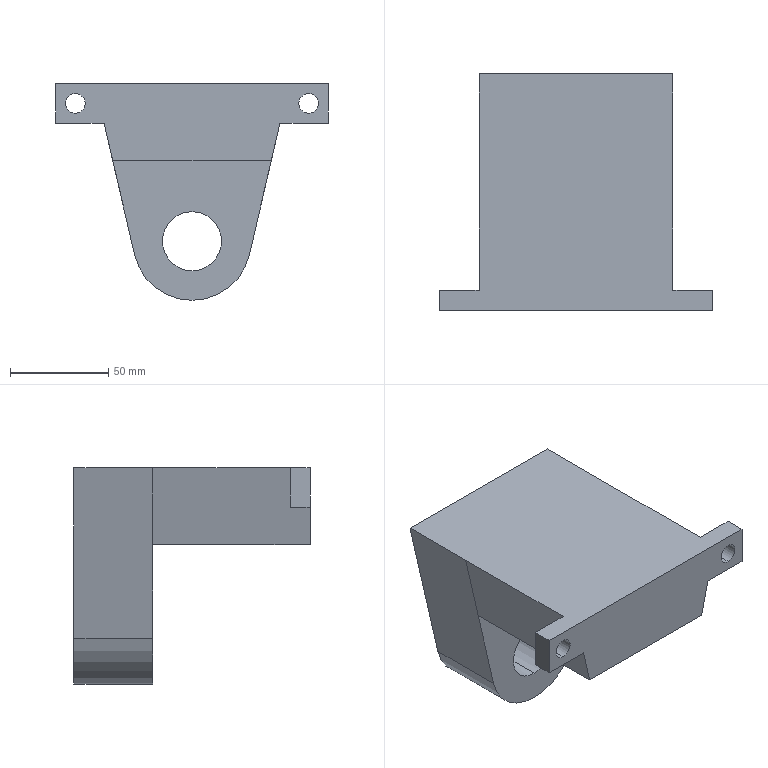Part | SolidWorks | features BaseBody 1 | 1 solid | 25 faces | box 138.517 x 120 x 109.993 mm | volume 571156 mm3 | plane 17 | cylinder 8 | commonest cylinder face diameters 10 x4 30 x2 59.986 x2
STEP:
#1=CARTESIAN_POINT('',(418.218,7.138,-275.));
#2=VERTEX_POINT('',#1);
#3=CARTESIAN_POINT('',(418.218,7.138,-285.));
#4=VERTEX_POINT('',#3);
#5=CARTESIAN_POINT('',(418.218,7.138,-280.));
#6=DIRECTION('',(0.,-1.,0.));
#7=DIRECTION('',(0.,0.,1.));
#8=AXIS2_PLACEMENT_3D('',#5,#6,#7);
#9=CIRCLE('',#8,5.);
#10=EDGE_CURVE('',#2,#4,#9,.T.);
#11=ORIENTED_EDGE('',*,*,#10,.T.);
#12=CARTESIAN_POINT('',(418.218,17.138,-285.));
#13=VERTEX_POINT('',#12);
#14=CARTESIAN_POINT('',(418.218,-2.862,-285.));
#15=DIRECTION('',(0.,1.,0.));
#16=VECTOR('',#15,1000.);
#17=LINE('',#14,#16);
#18=EDGE_CURVE('',#4,#13,#17,.T.);
#19=ORIENTED_EDGE('',*,*,#18,.T.);
#20=CARTESIAN_POINT('',(418.218,17.138,-275.));
#21=VERTEX_POINT('',#20);
#22=CARTESIAN_POINT('',(418.218,17.138,-280.));
#23=DIRECTION('',(0.,1.,0.));
#24=DIRECTION('',(0.,0.,1.));
#25=AXIS2_PLACEMENT_3D('',#22,#23,#24);
#26=CIRCLE('',#25,5.);
#27=EDGE_CURVE('',#13,#21,#26,.T.);
#28=ORIENTED_EDGE('',*,*,#27,.T.);
#29=CARTESIAN_POINT('',(418.218,-2.862,-275.));
#30=DIRECTION('',(0.,1.,0.));
#31=VECTOR('',#30,1000.);
#32=LINE('',#29,#31);
#33=EDGE_CURVE('',#2,#21,#32,.T.);
#34=ORIENTED_EDGE('',*,*,#33,.F.);
#35=EDGE_LOOP('',(#11,#19,#28,#34));
#36=FACE_OUTER_BOUND('',#35,.T.);
#37=CARTESIAN_POINT('',(418.218,-2.862,-280.));
#38=DIRECTION('',(0.,1.,0.));
#39=DIRECTION('',(0.,0.,1.));
#40=AXIS2_PLACEMENT_3D('',#37,#38,#39);
#41=CYLINDRICAL_SURFACE('',#40,5.);
#42=ADVANCED_FACE('',(#36),#41,.F.);
#43=CARTESIAN_POINT('',(299.701,7.138,-275.));
#44=VERTEX_POINT('',#43);
#45=CARTESIAN_POINT('',(299.701,7.138,-285.));
#46=VERTEX_POINT('',#45);
#47=CARTESIAN_POINT('',(299.701,7.138,-280.));
#48=DIRECTION('',(0.,-1.,0.));
#49=DIRECTION('',(0.,0.,1.));
#50=AXIS2_PLACEMENT_3D('',#47,#48,#49);
#51=CIRCLE('',#50,5.);
#52=EDGE_CURVE('',#44,#46,#51,.T.);
#53=ORIENTED_EDGE('',*,*,#52,.T.);
#54=CARTESIAN_POINT('',(299.701,17.138,-285.));
#55=VERTEX_POINT('',#54);
#56=CARTESIAN_POINT('',(299.701,-2.862,-285.));
#57=DIRECTION('',(0.,1.,0.));
#58=VECTOR('',#57,1000.);
#59=LINE('',#56,#58);
#60=EDGE_CURVE('',#46,#55,#59,.T.);
#61=ORIENTED_EDGE('',*,*,#60,.T.);
#62=CARTESIAN_POINT('',(299.701,17.138,-275.));
#63=VERTEX_POINT('',#62);
#64=CARTESIAN_POINT('',(299.701,17.138,-280.));
#65=DIRECTION('',(0.,1.,0.));
#66=DIRECTION('',(0.,0.,1.));
#67=AXIS2_PLACEMENT_3D('',#64,#65,#66);
#68=CIRCLE('',#67,5.);
#69=EDGE_CURVE('',#55,#63,#68,.T.);
#70=ORIENTED_EDGE('',*,*,#69,.T.);
#71=CARTESIAN_POINT('',(299.701,-2.862,-275.));
#72=DIRECTION('',(0.,1.,0.));
#73=VECTOR('',#72,1000.);
#74=LINE('',#71,#73);
#75=EDGE_CURVE('',#44,#63,#74,.T.);
#76=ORIENTED_EDGE('',*,*,#75,.F.);
#77=EDGE_LOOP('',(#53,#61,#70,#76));
#78=FACE_OUTER_BOUND('',#77,.T.);
#79=CARTESIAN_POINT('',(299.701,-2.862,-280.));
#80=DIRECTION('',(0.,1.,0.));
#81=DIRECTION('',(0.,0.,1.));
#82=AXIS2_PLACEMENT_3D('',#79,#80,#81);
#83=CYLINDRICAL_SURFACE('',#82,5.);
#84=ADVANCED_FACE('',(#78),#83,.F.);
#85=CARTESIAN_POINT('',(358.959,127.138,-379.993));
#86=VERTEX_POINT('',#85);
#87=CARTESIAN_POINT('',(329.736,127.138,-356.749));
#88=VERTEX_POINT('',#87);
#89=CARTESIAN_POINT('',(358.959,127.138,-350.));
#90=DIRECTION('',(0.,1.,0.));
#91=DIRECTION('',(0.,0.,1.));
#92=AXIS2_PLACEMENT_3D('',#89,#90,#91);
#93=CIRCLE('',#92,29.993);
#94=EDGE_CURVE('',#86,#88,#93,.T.);
#95=ORIENTED_EDGE('',*,*,#94,.F.);
#96=CARTESIAN_POINT('',(358.959,87.138,-379.993));
#97=VERTEX_POINT('',#96);
#98=CARTESIAN_POINT('',(358.959,127.138,-379.993));
#99=DIRECTION('',(0.,-1.,0.));
#100=VECTOR('',#99,1000.);
#101=LINE('',#98,#100);
#102=EDGE_CURVE('',#86,#97,#101,.T.);
#103=ORIENTED_EDGE('',*,*,#102,.T.);
#104=CARTESIAN_POINT('',(329.736,87.138,-356.749));
#105=VERTEX_POINT('',#104);
#106=CARTESIAN_POINT('',(358.959,87.138,-350.));
#107=DIRECTION('',(0.,1.,0.));
#108=DIRECTION('',(0.,0.,1.));
#109=AXIS2_PLACEMENT_3D('',#106,#107,#108);
#110=CIRCLE('',#109,29.993);
#111=EDGE_CURVE('',#97,#105,#110,.T.);
#112=ORIENTED_EDGE('',*,*,#111,.T.);
#113=CARTESIAN_POINT('',(329.736,127.138,-356.749));
#114=DIRECTION('',(0.,-1.,0.));
#115=VECTOR('',#114,1000.);
#116=LINE('',#113,#115);
#117=EDGE_CURVE('',#88,#105,#116,.T.);
#118=ORIENTED_EDGE('',*,*,#117,.F.);
#119=EDGE_LOOP('',(#95,#103,#112,#118));
#120=FACE_OUTER_BOUND('',#119,.T.);
#121=CARTESIAN_POINT('',(358.959,127.138,-350.));
#122=DIRECTION('',(0.,-1.,0.));
#123=DIRECTION('',(0.,0.,-1.));
#124=AXIS2_PLACEMENT_3D('',#121,#122,#123);
#125=CYLINDRICAL_SURFACE('',#124,29.993);
#126=ADVANCED_FACE('',(#120),#125,.T.);
#127=CARTESIAN_POINT('',(358.959,87.138,-365.));
#128=VERTEX_POINT('',#127);
#129=CARTESIAN_POINT('',(358.959,87.138,-335.));
#130=VERTEX_POINT('',#129);
#131=CARTESIAN_POINT('',(358.959,87.138,-350.));
#132=DIRECTION('',(0.,1.,0.));
#133=DIRECTION('',(0.,0.,1.));
#134=AXIS2_PLACEMENT_3D('',#131,#132,#133);
#135=CIRCLE('',#134,15.);
#136=EDGE_CURVE('',#128,#130,#135,.T.);
#137=ORIENTED_EDGE('',*,*,#136,.F.);
#138=CARTESIAN_POINT('',(358.959,127.138,-365.));
#139=VERTEX_POINT('',#138);
#140=CARTESIAN_POINT('',(358.959,87.138,-365.));
#141=DIRECTION('',(0.,1.,0.));
#142=VECTOR('',#141,1000.);
#143=LINE('',#140,#142);
#144=EDGE_CURVE('',#128,#139,#143,.T.);
#145=ORIENTED_EDGE('',*,*,#144,.T.);
#146=CARTESIAN_POINT('',(358.959,127.138,-335.));
#147=VERTEX_POINT('',#146);
#148=CARTESIAN_POINT('',(358.959,127.138,-350.));
#149=DIRECTION('',(0.,1.,0.));
#150=DIRECTION('',(0.,0.,1.));
#151=AXIS2_PLACEMENT_3D('',#148,#149,#150);
#152=CIRCLE('',#151,15.);
#153=EDGE_CURVE('',#139,#147,#152,.T.);
#154=ORIENTED_EDGE('',*,*,#153,.T.);
#155=CARTESIAN_POINT('',(358.959,87.138,-335.));
#156=DIRECTION('',(0.,1.,0.));
#157=VECTOR('',#156,1000.);
#158=LINE('',#155,#157);
#159=EDGE_CURVE('',#130,#147,#158,.T.);
#160=ORIENTED_EDGE('',*,*,#159,.F.);
#161=EDGE_LOOP('',(#137,#145,#154,#160));
#162=FACE_OUTER_BOUND('',#161,.T.);
#163=CARTESIAN_POINT('',(358.959,87.138,-350.));
#164=DIRECTION('',(0.,1.,0.));
#165=DIRECTION('',(0.,0.,1.));
#166=AXIS2_PLACEMENT_3D('',#163,#164,#165);
#167=CYLINDRICAL_SURFACE('',#166,15.);
#168=ADVANCED_FACE('',(#162),#167,.F.);
#169=ORIENTED_EDGE('',*,*,#144,.F.);
#170=CARTESIAN_POINT('',(358.959,87.138,-350.));
#171=DIRECTION('',(0.,1.,0.));
#172=DIRECTION('',(0.,0.,1.));
#173=AXIS2_PLACEMENT_3D('',#170,#171,#172);
#174=CIRCLE('',#173,15.);
#175=EDGE_CURVE('',#130,#128,#174,.T.);
#176=ORIENTED_EDGE('',*,*,#175,.F.);
#177=ORIENTED_EDGE('',*,*,#159,.T.);
#178=CARTESIAN_POINT('',(358.959,127.138,-350.));
#179=DIRECTION('',(0.,1.,0.));
#180=DIRECTION('',(0.,0.,1.));
#181=AXIS2_PLACEMENT_3D('',#178,#179,#180);
#182=CIRCLE('',#181,15.);
#183=EDGE_CURVE('',#147,#139,#182,.T.);
#184=ORIENTED_EDGE('',*,*,#183,.T.);
#185=EDGE_LOOP('',(#169,#176,#177,#184));
#186=FACE_OUTER_BOUND('',#185,.T.);
#187=CARTESIAN_POINT('',(358.959,87.138,-350.));
#188=DIRECTION('',(0.,1.,0.));
#189=DIRECTION('',(0.,0.,1.));
#190=AXIS2_PLACEMENT_3D('',#187,#188,#189);
#191=CYLINDRICAL_SURFACE('',#190,15.);
#192=ADVANCED_FACE('',(#186),#191,.F.);
#193=ORIENTED_EDGE('',*,*,#102,.F.);
#194=CARTESIAN_POINT('',(388.183,127.138,-356.749));
#195=VERTEX_POINT('',#194);
#196=CARTESIAN_POINT('',(358.959,127.138,-350.));
#197=DIRECTION('',(0.,1.,0.));
#198=DIRECTION('',(0.,0.,1.));
#199=AXIS2_PLACEMENT_3D('',#196,#197,#198);
#200=CIRCLE('',#199,29.993);
#201=EDGE_CURVE('',#195,#86,#200,.T.);
#202=ORIENTED_EDGE('',*,*,#201,.F.);
#203=CARTESIAN_POINT('',(388.183,87.138,-356.749));
#204=VERTEX_POINT('',#203);
#205=CARTESIAN_POINT('',(388.183,127.138,-356.749));
#206=DIRECTION('',(0.,-1.,0.));
#207=VECTOR('',#206,1000.);
#208=LINE('',#205,#207);
#209=EDGE_CURVE('',#195,#204,#208,.T.);
#210=ORIENTED_EDGE('',*,*,#209,.T.);
#211=CARTESIAN_POINT('',(358.959,87.138,-350.));
#212=DIRECTION('',(0.,1.,0.));
#213=DIRECTION('',(0.,0.,1.));
#214=AXIS2_PLACEMENT_3D('',#211,#212,#213);
#215=CIRCLE('',#214,29.993);
#216=EDGE_CURVE('',#204,#97,#215,.T.);
#217=ORIENTED_EDGE('',*,*,#216,.T.);
#218=EDGE_LOOP('',(#193,#202,#210,#217));
#219=FACE_OUTER_BOUND('',#218,.T.);
#220=CARTESIAN_POINT('',(358.959,127.138,-350.));
#221=DIRECTION('',(0.,-1.,0.));
#222=DIRECTION('',(0.,0.,-1.));
#223=AXIS2_PLACEMENT_3D('',#220,#221,#222);
#224=CYLINDRICAL_SURFACE('',#223,29.993);
#225=ADVANCED_FACE('',(#219),#224,.T.);
#226=CARTESIAN_POINT('',(408.218,87.138,-270.));
#227=VERTEX_POINT('',#226);
#228=CARTESIAN_POINT('',(399.211,87.138,-309.));
#229=VERTEX_POINT('',#228);
#230=CARTESIAN_POINT('',(408.218,87.138,-270.));
#231=DIRECTION('',(-0.225,0.,-0.9744));
#232=VECTOR('',#231,1000.);
#233=LINE('',#230,#232);
#234=EDGE_CURVE('',#227,#229,#233,.T.);
#235=ORIENTED_EDGE('',*,*,#234,.F.);
#236=CARTESIAN_POINT('',(399.214,87.138,-309.));
#237=VERTEX_POINT('',#236);
#238=CARTESIAN_POINT('',(408.218,87.138,-270.));
#239=DIRECTION('',(-0.225,0.,-0.9744));
#240=VECTOR('',#239,1000.);
#241=LINE('',#238,#240);
#242=EDGE_CURVE('',#227,#237,#241,.T.);
#243=ORIENTED_EDGE('',*,*,#242,.T.);
#244=CARTESIAN_POINT('',(318.704,87.138,-309.));
#245=DIRECTION('',(-1.,0.,0.));
#246=VECTOR('',#245,1000.);
#247=LINE('',#244,#246);
#248=EDGE_CURVE('',#237,#229,#247,.T.);
#249=ORIENTED_EDGE('',*,*,#248,.T.);
#250=EDGE_LOOP('',(#235,#243,#249));
#251=FACE_OUTER_BOUND('',#250,.T.);
#252=CARTESIAN_POINT('',(-616.782,87.138,0.));
#253=DIRECTION('',(0.,-1.,0.));
#254=DIRECTION('',(0.,0.,-1.));
#255=AXIS2_PLACEMENT_3D('',#252,#253,#254);
#256=PLANE('',#255);
#257=ADVANCED_FACE('',(#251),#256,.F.);
#258=ORIENTED_EDGE('',*,*,#175,.T.);
#259=ORIENTED_EDGE('',*,*,#136,.T.);
#260=EDGE_LOOP('',(#258,#259));
#261=FACE_BOUND('',#260,.T.);
#262=CARTESIAN_POINT('',(408.218,87.138,-270.));
#263=DIRECTION('',(-0.225,0.,-0.9744));
#264=VECTOR('',#263,1000.);
#265=LINE('',#262,#264);
#266=EDGE_CURVE('',#229,#204,#265,.T.);
#267=ORIENTED_EDGE('',*,*,#266,.F.);
#268=CARTESIAN_POINT('',(318.708,87.138,-309.));
#269=VERTEX_POINT('',#268);
#270=CARTESIAN_POINT('',(318.704,87.138,-309.));
#271=DIRECTION('',(-1.,0.,0.));
#272=VECTOR('',#271,1000.);
#273=LINE('',#270,#272);
#274=EDGE_CURVE('',#229,#269,#273,.T.);
#275=ORIENTED_EDGE('',*,*,#274,.T.);
#276=CARTESIAN_POINT('',(309.701,87.138,-270.));
#277=DIRECTION('',(-0.225,0.,0.9744));
#278=VECTOR('',#277,1000.);
#279=LINE('',#276,#278);
#280=EDGE_CURVE('',#105,#269,#279,.T.);
#281=ORIENTED_EDGE('',*,*,#280,.F.);
#282=ORIENTED_EDGE('',*,*,#111,.F.);
#283=ORIENTED_EDGE('',*,*,#216,.F.);
#284=EDGE_LOOP('',(#267,#275,#281,#282,#283));
#285=FACE_OUTER_BOUND('',#284,.T.);
#286=CARTESIAN_POINT('',(358.959,87.138,-350.));
#287=DIRECTION('',(0.,1.,0.));
#288=DIRECTION('',(0.,0.,1.));
#289=AXIS2_PLACEMENT_3D('',#286,#287,#288);
#290=PLANE('',#289);
#291=ADVANCED_FACE('',(#261,#285),#290,.F.);
#292=CARTESIAN_POINT('',(309.701,87.138,-270.));
#293=VERTEX_POINT('',#292);
#294=CARTESIAN_POINT('',(309.701,87.138,-270.));
#295=DIRECTION('',(-0.225,0.,0.9744));
#296=VECTOR('',#295,1000.);
#297=LINE('',#294,#296);
#298=EDGE_CURVE('',#269,#293,#297,.T.);
#299=ORIENTED_EDGE('',*,*,#298,.F.);
#300=CARTESIAN_POINT('',(318.704,87.138,-309.));
#301=VERTEX_POINT('',#300);
#302=CARTESIAN_POINT('',(318.704,87.138,-309.));
#303=DIRECTION('',(-1.,0.,0.));
#304=VECTOR('',#303,1000.);
#305=LINE('',#302,#304);
#306=EDGE_CURVE('',#269,#301,#305,.T.);
#307=ORIENTED_EDGE('',*,*,#306,.T.);
#308=CARTESIAN_POINT('',(309.701,87.138,-270.));
#309=DIRECTION('',(-0.225,0.,0.9744));
#310=VECTOR('',#309,1000.);
#311=LINE('',#308,#310);
#312=EDGE_CURVE('',#301,#293,#311,.T.);
#313=ORIENTED_EDGE('',*,*,#312,.T.);
#314=EDGE_LOOP('',(#299,#307,#313));
#315=FACE_OUTER_BOUND('',#314,.T.);
#316=CARTESIAN_POINT('',(-616.782,87.138,0.));
#317=DIRECTION('',(0.,-1.,0.));
#318=DIRECTION('',(0.,0.,-1.));
#319=AXIS2_PLACEMENT_3D('',#316,#317,#318);
#320=PLANE('',#319);
#321=ADVANCED_FACE('',(#315),#320,.F.);
#322=ORIENTED_EDGE('',*,*,#280,.T.);
#323=ORIENTED_EDGE('',*,*,#298,.T.);
#324=CARTESIAN_POINT('',(309.701,127.138,-270.));
#325=VERTEX_POINT('',#324);
#326=CARTESIAN_POINT('',(309.701,127.138,-270.));
#327=DIRECTION('',(0.,-1.,0.));
#328=VECTOR('',#327,1000.);
#329=LINE('',#326,#328);
#330=EDGE_CURVE('',#325,#293,#329,.T.);
#331=ORIENTED_EDGE('',*,*,#330,.F.);
#332=CARTESIAN_POINT('',(309.701,127.138,-270.));
#333=DIRECTION('',(-0.225,0.,0.9744));
#334=VECTOR('',#333,1000.);
#335=LINE('',#332,#334);
#336=EDGE_CURVE('',#88,#325,#335,.T.);
#337=ORIENTED_EDGE('',*,*,#336,.F.);
#338=ORIENTED_EDGE('',*,*,#117,.T.);
#339=EDGE_LOOP('',(#322,#323,#331,#337,#338));
#340=FACE_OUTER_BOUND('',#339,.T.);
#341=CARTESIAN_POINT('',(309.701,127.138,-270.));
#342=DIRECTION('',(0.9744,0.,0.225));
#343=DIRECTION('',(0.225,0.,-0.9744));
#344=AXIS2_PLACEMENT_3D('',#341,#342,#343);
#345=PLANE('',#344);
#346=ADVANCED_FACE('',(#340),#345,.F.);
#347=ORIENTED_EDGE('',*,*,#183,.F.);
#348=ORIENTED_EDGE('',*,*,#153,.F.);
#349=EDGE_LOOP('',(#347,#348));
#350=FACE_BOUND('',#349,.T.);
#351=ORIENTED_EDGE('',*,*,#336,.T.);
#352=CARTESIAN_POINT('',(408.218,127.138,-270.));
#353=VERTEX_POINT('',#352);
#354=CARTESIAN_POINT('',(309.701,127.138,-270.));
#355=DIRECTION('',(1.,0.,0.));
#356=VECTOR('',#355,1000.);
#357=LINE('',#354,#356);
#358=EDGE_CURVE('',#325,#353,#357,.T.);
#359=ORIENTED_EDGE('',*,*,#358,.T.);
#360=CARTESIAN_POINT('',(408.218,127.138,-270.));
#361=DIRECTION('',(-0.225,0.,-0.9744));
#362=VECTOR('',#361,1000.);
#363=LINE('',#360,#362);
#364=EDGE_CURVE('',#353,#195,#363,.T.);
#365=ORIENTED_EDGE('',*,*,#364,.T.);
#366=ORIENTED_EDGE('',*,*,#201,.T.);
#367=ORIENTED_EDGE('',*,*,#94,.T.);
#368=EDGE_LOOP('',(#351,#359,#365,#366,#367));
#369=FACE_OUTER_BOUND('',#368,.T.);
#370=CARTESIAN_POINT('',(358.959,127.138,-350.));
#371=DIRECTION('',(0.,1.,0.));
#372=DIRECTION('',(0.,0.,1.));
#373=AXIS2_PLACEMENT_3D('',#370,#371,#372);
#374=PLANE('',#373);
#375=ADVANCED_FACE('',(#350,#369),#374,.T.);
#376=ORIENTED_EDGE('',*,*,#234,.T.);
#377=ORIENTED_EDGE('',*,*,#266,.T.);
#378=ORIENTED_EDGE('',*,*,#209,.F.);
#379=ORIENTED_EDGE('',*,*,#364,.F.);
#380=CARTESIAN_POINT('',(408.218,127.138,-270.));
#381=DIRECTION('',(0.,-1.,0.));
#382=VECTOR('',#381,1000.);
#383=LINE('',#380,#382);
#384=EDGE_CURVE('',#353,#227,#383,.T.);
#385=ORIENTED_EDGE('',*,*,#384,.T.);
#386=EDGE_LOOP('',(#376,#377,#378,#379,#385));
#387=FACE_OUTER_BOUND('',#386,.T.);
#388=CARTESIAN_POINT('',(408.218,127.138,-270.));
#389=DIRECTION('',(-0.9744,0.,0.225));
#390=DIRECTION('',(0.225,0.,0.9744));
#391=AXIS2_PLACEMENT_3D('',#388,#389,#390);
#392=PLANE('',#391);
#393=ADVANCED_FACE('',(#387),#392,.F.);
#394=CARTESIAN_POINT('',(399.214,7.138,-309.));
#395=VERTEX_POINT('',#394);
#396=CARTESIAN_POINT('',(399.214,87.138,-309.));
#397=DIRECTION('',(0.,-1.,0.));
#398=VECTOR('',#397,1000.);
#399=LINE('',#396,#398);
#400=EDGE_CURVE('',#237,#395,#399,.T.);
#401=ORIENTED_EDGE('',*,*,#400,.T.);
#402=CARTESIAN_POINT('',(318.704,7.138,-309.));
#403=VERTEX_POINT('',#402);
#404=CARTESIAN_POINT('',(192.218,7.138,-309.));
#405=DIRECTION('',(-1.,0.,0.));
#406=VECTOR('',#405,1000.);
#407=LINE('',#404,#406);
#408=EDGE_CURVE('',#395,#403,#407,.T.);
#409=ORIENTED_EDGE('',*,*,#408,.T.);
#410=CARTESIAN_POINT('',(318.704,87.138,-309.));
#411=DIRECTION('',(0.,-1.,0.));
#412=VECTOR('',#411,1000.);
#413=LINE('',#410,#412);
#414=EDGE_CURVE('',#301,#403,#413,.T.);
#415=ORIENTED_EDGE('',*,*,#414,.F.);
#416=ORIENTED_EDGE('',*,*,#306,.F.);
#417=ORIENTED_EDGE('',*,*,#274,.F.);
#418=ORIENTED_EDGE('',*,*,#248,.F.);
#419=EDGE_LOOP('',(#401,#409,#415,#416,#417,#418));
#420=FACE_OUTER_BOUND('',#419,.T.);
#421=CARTESIAN_POINT('',(192.218,7.138,-309.));
#422=DIRECTION('',(0.,0.,1.));
#423=DIRECTION('',(1.,0.,0.));
#424=AXIS2_PLACEMENT_3D('',#421,#422,#423);
#425=PLANE('',#424);
#426=ADVANCED_FACE('',(#420),#425,.F.);
#427=CARTESIAN_POINT('',(289.701,7.138,-290.));
#428=VERTEX_POINT('',#427);
#429=CARTESIAN_POINT('',(289.701,7.138,-270.));
#430=VERTEX_POINT('',#429);
#431=CARTESIAN_POINT('',(289.701,7.138,-270.));
#432=DIRECTION('',(0.,0.,1.));
#433=VECTOR('',#432,1000.);
#434=LINE('',#431,#433);
#435=EDGE_CURVE('',#428,#430,#434,.T.);
#436=ORIENTED_EDGE('',*,*,#435,.T.);
#437=CARTESIAN_POINT('',(289.701,17.138,-270.));
#438=VERTEX_POINT('',#437);
#439=CARTESIAN_POINT('',(289.701,17.138,-270.));
#440=DIRECTION('',(0.,-1.,0.));
#441=VECTOR('',#440,1000.);
#442=LINE('',#439,#441);
#443=EDGE_CURVE('',#438,#430,#442,.T.);
#444=ORIENTED_EDGE('',*,*,#443,.F.);
#445=CARTESIAN_POINT('',(289.701,17.138,-290.));
#446=VERTEX_POINT('',#445);
#447=CARTESIAN_POINT('',(289.701,17.138,-270.));
#448=DIRECTION('',(0.,0.,1.));
#449=VECTOR('',#448,1000.);
#450=LINE('',#447,#449);
#451=EDGE_CURVE('',#446,#438,#450,.T.);
#452=ORIENTED_EDGE('',*,*,#451,.F.);
#453=CARTESIAN_POINT('',(289.701,17.138,-290.));
#454=DIRECTION('',(0.,-1.,0.));
#455=VECTOR('',#454,1000.);
#456=LINE('',#453,#455);
#457=EDGE_CURVE('',#446,#428,#456,.T.);
#458=ORIENTED_EDGE('',*,*,#457,.T.);
#459=EDGE_LOOP('',(#436,#444,#452,#458));
#460=FACE_OUTER_BOUND('',#459,.T.);
#461=CARTESIAN_POINT('',(289.701,17.138,-270.));
#462=DIRECTION('',(1.,0.,0.));
#463=DIRECTION('',(0.,0.,-1.));
#464=AXIS2_PLACEMENT_3D('',#461,#462,#463);
#465=PLANE('',#464);
#466=ADVANCED_FACE('',(#460),#465,.F.);
#467=CARTESIAN_POINT('',(314.318,7.138,-290.));
#468=VERTEX_POINT('',#467);
#469=CARTESIAN_POINT('',(289.701,7.138,-290.));
#470=DIRECTION('',(-1.,0.,0.));
#471=VECTOR('',#470,1000.);
#472=LINE('',#469,#471);
#473=EDGE_CURVE('',#468,#428,#472,.T.);
#474=ORIENTED_EDGE('',*,*,#473,.T.);
#475=ORIENTED_EDGE('',*,*,#457,.F.);
#476=CARTESIAN_POINT('',(314.318,17.138,-290.));
#477=VERTEX_POINT('',#476);
#478=CARTESIAN_POINT('',(289.701,17.138,-290.));
#479=DIRECTION('',(-1.,0.,0.));
#480=VECTOR('',#479,1000.);
#481=LINE('',#478,#480);
#482=EDGE_CURVE('',#477,#446,#481,.T.);
#483=ORIENTED_EDGE('',*,*,#482,.F.);
#484=CARTESIAN_POINT('',(314.318,17.138,-290.));
#485=DIRECTION('',(0.,-1.,0.));
#486=VECTOR('',#485,1000.);
#487=LINE('',#484,#486);
#488=EDGE_CURVE('',#477,#468,#487,.T.);
#489=ORIENTED_EDGE('',*,*,#488,.T.);
#490=EDGE_LOOP('',(#474,#475,#483,#489));
#491=FACE_OUTER_BOUND('',#490,.T.);
#492=CARTESIAN_POINT('',(289.701,17.138,-290.));
#493=DIRECTION('',(0.,0.,1.));
#494=DIRECTION('',(1.,0.,0.));
#495=AXIS2_PLACEMENT_3D('',#492,#493,#494);
#496=PLANE('',#495);
#497=ADVANCED_FACE('',(#491),#496,.F.);
#498=CARTESIAN_POINT('',(428.218,7.138,-290.));
#499=VERTEX_POINT('',#498);
#500=CARTESIAN_POINT('',(403.6,7.138,-290.));
#501=VERTEX_POINT('',#500);
#502=CARTESIAN_POINT('',(428.218,7.138,-290.));
#503=DIRECTION('',(-1.,0.,0.));
#504=VECTOR('',#503,1000.);
#505=LINE('',#502,#504);
#506=EDGE_CURVE('',#499,#501,#505,.T.);
#507=ORIENTED_EDGE('',*,*,#506,.T.);
#508=CARTESIAN_POINT('',(403.6,17.138,-290.));
#509=VERTEX_POINT('',#508);
#510=CARTESIAN_POINT('',(403.6,17.138,-290.));
#511=DIRECTION('',(0.,-1.,0.));
#512=VECTOR('',#511,1000.);
#513=LINE('',#510,#512);
#514=EDGE_CURVE('',#509,#501,#513,.T.);
#515=ORIENTED_EDGE('',*,*,#514,.F.);
#516=CARTESIAN_POINT('',(428.218,17.138,-290.));
#517=VERTEX_POINT('',#516);
#518=CARTESIAN_POINT('',(428.218,17.138,-290.));
#519=DIRECTION('',(-1.,0.,0.));
#520=VECTOR('',#519,1000.);
#521=LINE('',#518,#520);
#522=EDGE_CURVE('',#517,#509,#521,.T.);
#523=ORIENTED_EDGE('',*,*,#522,.F.);
#524=CARTESIAN_POINT('',(428.218,17.138,-290.));
#525=DIRECTION('',(0.,-1.,0.));
#526=VECTOR('',#525,1000.);
#527=LINE('',#524,#526);
#528=EDGE_CURVE('',#517,#499,#527,.T.);
#529=ORIENTED_EDGE('',*,*,#528,.T.);
#530=EDGE_LOOP('',(#507,#515,#523,#529));
#531=FACE_OUTER_BOUND('',#530,.T.);
#532=CARTESIAN_POINT('',(428.218,17.138,-290.));
#533=DIRECTION('',(0.,0.,1.));
#534=DIRECTION('',(1.,0.,0.));
#535=AXIS2_PLACEMENT_3D('',#532,#533,#534);
#536=PLANE('',#535);
#537=ADVANCED_FACE('',(#531),#536,.F.);
#538=CARTESIAN_POINT('',(428.218,7.138,-270.));
#539=VERTEX_POINT('',#538);
#540=CARTESIAN_POINT('',(428.218,7.138,-270.));
#541=DIRECTION('',(0.,0.,-1.));
#542=VECTOR('',#541,1000.);
#543=LINE('',#540,#542);
#544=EDGE_CURVE('',#539,#499,#543,.T.);
#545=ORIENTED_EDGE('',*,*,#544,.T.);
#546=ORIENTED_EDGE('',*,*,#528,.F.);
#547=CARTESIAN_POINT('',(428.218,17.138,-270.));
#548=VERTEX_POINT('',#547);
#549=CARTESIAN_POINT('',(428.218,17.138,-270.));
#550=DIRECTION('',(0.,0.,-1.));
#551=VECTOR('',#550,1000.);
#552=LINE('',#549,#551);
#553=EDGE_CURVE('',#548,#517,#552,.T.);
#554=ORIENTED_EDGE('',*,*,#553,.F.);
#555=CARTESIAN_POINT('',(428.218,17.138,-270.));
#556=DIRECTION('',(0.,-1.,0.));
#557=VECTOR('',#556,1000.);
#558=LINE('',#555,#557);
#559=EDGE_CURVE('',#548,#539,#558,.T.);
#560=ORIENTED_EDGE('',*,*,#559,.T.);
#561=EDGE_LOOP('',(#545,#546,#554,#560));
#562=FACE_OUTER_BOUND('',#561,.T.);
#563=CARTESIAN_POINT('',(428.218,17.138,-270.));
#564=DIRECTION('',(-1.,0.,0.));
#565=DIRECTION('',(0.,0.,1.));
#566=AXIS2_PLACEMENT_3D('',#563,#564,#565);
#567=PLANE('',#566);
#568=ADVANCED_FACE('',(#562),#567,.F.);
#569=CARTESIAN_POINT('',(309.701,7.138,-270.));
#570=DIRECTION('',(1.,0.,0.));
#571=VECTOR('',#570,1000.);
#572=LINE('',#569,#571);
#573=EDGE_CURVE('',#430,#539,#572,.T.);
#574=ORIENTED_EDGE('',*,*,#573,.T.);
#575=ORIENTED_EDGE('',*,*,#559,.F.);
#576=CARTESIAN_POINT('',(408.218,17.138,-270.));
#577=VERTEX_POINT('',#576);
#578=CARTESIAN_POINT('',(408.218,17.138,-270.));
#579=DIRECTION('',(1.,0.,0.));
#580=VECTOR('',#579,1000.);
#581=LINE('',#578,#580);
#582=EDGE_CURVE('',#577,#548,#581,.T.);
#583=ORIENTED_EDGE('',*,*,#582,.F.);
#584=CARTESIAN_POINT('',(408.218,87.138,-270.));
#585=DIRECTION('',(0.,-1.,0.));
#586=VECTOR('',#585,1000.);
#587=LINE('',#584,#586);
#588=EDGE_CURVE('',#227,#577,#587,.T.);
#589=ORIENTED_EDGE('',*,*,#588,.F.);
#590=ORIENTED_EDGE('',*,*,#384,.F.);
#591=ORIENTED_EDGE('',*,*,#358,.F.);
#592=ORIENTED_EDGE('',*,*,#330,.T.);
#593=CARTESIAN_POINT('',(309.701,17.138,-270.));
#594=VERTEX_POINT('',#593);
#595=CARTESIAN_POINT('',(309.701,87.138,-270.));
#596=DIRECTION('',(0.,-1.,0.));
#597=VECTOR('',#596,1000.);
#598=LINE('',#595,#597);
#599=EDGE_CURVE('',#293,#594,#598,.T.);
#600=ORIENTED_EDGE('',*,*,#599,.T.);
#601=CARTESIAN_POINT('',(309.701,17.138,-270.));
#602=DIRECTION('',(1.,0.,0.));
#603=VECTOR('',#602,1000.);
#604=LINE('',#601,#603);
#605=EDGE_CURVE('',#438,#594,#604,.T.);
#606=ORIENTED_EDGE('',*,*,#605,.F.);
#607=ORIENTED_EDGE('',*,*,#443,.T.);
#608=EDGE_LOOP('',(#574,#575,#583,#589,#590,#591,#592,#600,#606,#607));
#609=FACE_OUTER_BOUND('',#608,.T.);
#610=CARTESIAN_POINT('',(309.701,87.138,-270.));
#611=DIRECTION('',(0.,0.,-1.));
#612=DIRECTION('',(-1.,0.,0.));
#613=AXIS2_PLACEMENT_3D('',#610,#611,#612);
#614=PLANE('',#613);
#615=ADVANCED_FACE('',(#609),#614,.F.);
#616=ORIENTED_EDGE('',*,*,#514,.T.);
#617=CARTESIAN_POINT('',(408.218,7.138,-270.));
#618=DIRECTION('',(-0.225,0.,-0.9744));
#619=VECTOR('',#618,1000.);
#620=LINE('',#617,#619);
#621=EDGE_CURVE('',#501,#395,#620,.T.);
#622=ORIENTED_EDGE('',*,*,#621,.T.);
#623=ORIENTED_EDGE('',*,*,#400,.F.);
#624=ORIENTED_EDGE('',*,*,#242,.F.);
#625=ORIENTED_EDGE('',*,*,#588,.T.);
#626=CARTESIAN_POINT('',(403.6,17.138,-290.));
#627=DIRECTION('',(0.225,0.,0.9744));
#628=VECTOR('',#627,1000.);
#629=LINE('',#626,#628);
#630=EDGE_CURVE('',#509,#577,#629,.T.);
#631=ORIENTED_EDGE('',*,*,#630,.F.);
#632=EDGE_LOOP('',(#616,#622,#623,#624,#625,#631));
#633=FACE_OUTER_BOUND('',#632,.T.);
#634=CARTESIAN_POINT('',(408.218,87.138,-270.));
#635=DIRECTION('',(-0.9744,0.,0.225));
#636=DIRECTION('',(0.225,0.,0.9744));
#637=AXIS2_PLACEMENT_3D('',#634,#635,#636);
#638=PLANE('',#637);
#639=ADVANCED_FACE('',(#633),#638,.F.);
#640=ORIENTED_EDGE('',*,*,#488,.F.);
#641=CARTESIAN_POINT('',(314.318,17.138,-290.));
#642=DIRECTION('',(0.225,0.,-0.9744));
#643=VECTOR('',#642,1000.);
#644=LINE('',#641,#643);
#645=EDGE_CURVE('',#594,#477,#644,.T.);
#646=ORIENTED_EDGE('',*,*,#645,.F.);
#647=ORIENTED_EDGE('',*,*,#599,.F.);
#648=ORIENTED_EDGE('',*,*,#312,.F.);
#649=ORIENTED_EDGE('',*,*,#414,.T.);
#650=CARTESIAN_POINT('',(309.701,7.138,-270.));
#651=DIRECTION('',(-0.225,0.,0.9744));
#652=VECTOR('',#651,1000.);
#653=LINE('',#650,#652);
#654=EDGE_CURVE('',#403,#468,#653,.T.);
#655=ORIENTED_EDGE('',*,*,#654,.T.);
#656=EDGE_LOOP('',(#640,#646,#647,#648,#649,#655));
#657=FACE_OUTER_BOUND('',#656,.T.);
#658=CARTESIAN_POINT('',(309.701,87.138,-270.));
#659=DIRECTION('',(0.9744,0.,0.225));
#660=DIRECTION('',(0.225,0.,-0.9744));
#661=AXIS2_PLACEMENT_3D('',#658,#659,#660);
#662=PLANE('',#661);
#663=ADVANCED_FACE('',(#657),#662,.F.);
#664=CARTESIAN_POINT('',(299.701,17.138,-280.));
#665=DIRECTION('',(0.,1.,0.));
#666=DIRECTION('',(0.,0.,1.));
#667=AXIS2_PLACEMENT_3D('',#664,#665,#666);
#668=CIRCLE('',#667,5.);
#669=EDGE_CURVE('',#63,#55,#668,.T.);
#670=ORIENTED_EDGE('',*,*,#669,.F.);
#671=ORIENTED_EDGE('',*,*,#69,.F.);
#672=EDGE_LOOP('',(#670,#671));
#673=FACE_BOUND('',#672,.T.);
#674=ORIENTED_EDGE('',*,*,#482,.T.);
#675=ORIENTED_EDGE('',*,*,#451,.T.);
#676=ORIENTED_EDGE('',*,*,#605,.T.);
#677=ORIENTED_EDGE('',*,*,#645,.T.);
#678=EDGE_LOOP('',(#674,#675,#676,#677));
#679=FACE_OUTER_BOUND('',#678,.T.);
#680=CARTESIAN_POINT('',(-616.782,17.138,0.));
#681=DIRECTION('',(0.,1.,0.));
#682=DIRECTION('',(0.,0.,1.));
#683=AXIS2_PLACEMENT_3D('',#680,#681,#682);
#684=PLANE('',#683);
#685=ADVANCED_FACE('',(#673,#679),#684,.T.);
#686=ORIENTED_EDGE('',*,*,#60,.F.);
#687=CARTESIAN_POINT('',(299.701,7.138,-280.));
#688=DIRECTION('',(0.,-1.,0.));
#689=DIRECTION('',(0.,0.,1.));
#690=AXIS2_PLACEMENT_3D('',#687,#688,#689);
#691=CIRCLE('',#690,5.);
#692=EDGE_CURVE('',#46,#44,#691,.T.);
#693=ORIENTED_EDGE('',*,*,#692,.T.);
#694=ORIENTED_EDGE('',*,*,#75,.T.);
#695=ORIENTED_EDGE('',*,*,#669,.T.);
#696=EDGE_LOOP('',(#686,#693,#694,#695));
#697=FACE_OUTER_BOUND('',#696,.T.);
#698=CARTESIAN_POINT('',(299.701,-2.862,-280.));
#699=DIRECTION('',(0.,1.,0.));
#700=DIRECTION('',(0.,0.,1.));
#701=AXIS2_PLACEMENT_3D('',#698,#699,#700);
#702=CYLINDRICAL_SURFACE('',#701,5.);
#703=ADVANCED_FACE('',(#697),#702,.F.);
#704=CARTESIAN_POINT('',(418.218,17.138,-280.));
#705=DIRECTION('',(0.,1.,0.));
#706=DIRECTION('',(0.,0.,1.));
#707=AXIS2_PLACEMENT_3D('',#704,#705,#706);
#708=CIRCLE('',#707,5.);
#709=EDGE_CURVE('',#21,#13,#708,.T.);
#710=ORIENTED_EDGE('',*,*,#709,.F.);
#711=ORIENTED_EDGE('',*,*,#27,.F.);
#712=EDGE_LOOP('',(#710,#711));
#713=FACE_BOUND('',#712,.T.);
#714=ORIENTED_EDGE('',*,*,#630,.T.);
#715=ORIENTED_EDGE('',*,*,#582,.T.);
#716=ORIENTED_EDGE('',*,*,#553,.T.);
#717=ORIENTED_EDGE('',*,*,#522,.T.);
#718=EDGE_LOOP('',(#714,#715,#716,#717));
#719=FACE_OUTER_BOUND('',#718,.T.);
#720=CARTESIAN_POINT('',(-616.782,17.138,0.));
#721=DIRECTION('',(0.,1.,0.));
#722=DIRECTION('',(0.,0.,1.));
#723=AXIS2_PLACEMENT_3D('',#720,#721,#722);
#724=PLANE('',#723);
#725=ADVANCED_FACE('',(#713,#719),#724,.T.);
#726=ORIENTED_EDGE('',*,*,#18,.F.);
#727=CARTESIAN_POINT('',(418.218,7.138,-280.));
#728=DIRECTION('',(0.,-1.,0.));
#729=DIRECTION('',(0.,0.,1.));
#730=AXIS2_PLACEMENT_3D('',#727,#728,#729);
#731=CIRCLE('',#730,5.);
#732=EDGE_CURVE('',#4,#2,#731,.T.);
#733=ORIENTED_EDGE('',*,*,#732,.T.);
#734=ORIENTED_EDGE('',*,*,#33,.T.);
#735=ORIENTED_EDGE('',*,*,#709,.T.);
#736=EDGE_LOOP('',(#726,#733,#734,#735));
#737=FACE_OUTER_BOUND('',#736,.T.);
#738=CARTESIAN_POINT('',(418.218,-2.862,-280.));
#739=DIRECTION('',(0.,1.,0.));
#740=DIRECTION('',(0.,0.,1.));
#741=AXIS2_PLACEMENT_3D('',#738,#739,#740);
#742=CYLINDRICAL_SURFACE('',#741,5.);
#743=ADVANCED_FACE('',(#737),#742,.F.);
#744=ORIENTED_EDGE('',*,*,#10,.F.);
#745=ORIENTED_EDGE('',*,*,#732,.F.);
#746=EDGE_LOOP('',(#744,#745));
#747=FACE_BOUND('',#746,.T.);
#748=ORIENTED_EDGE('',*,*,#52,.F.);
#749=ORIENTED_EDGE('',*,*,#692,.F.);
#750=EDGE_LOOP('',(#748,#749));
#751=FACE_BOUND('',#750,.T.);
#752=ORIENTED_EDGE('',*,*,#573,.F.);
#753=ORIENTED_EDGE('',*,*,#435,.F.);
#754=ORIENTED_EDGE('',*,*,#473,.F.);
#755=ORIENTED_EDGE('',*,*,#654,.F.);
#756=ORIENTED_EDGE('',*,*,#408,.F.);
#757=ORIENTED_EDGE('',*,*,#621,.F.);
#758=ORIENTED_EDGE('',*,*,#506,.F.);
#759=ORIENTED_EDGE('',*,*,#544,.F.);
#760=EDGE_LOOP('',(#752,#753,#754,#755,#756,#757,#758,#759));
#761=FACE_OUTER_BOUND('',#760,.T.);
#762=CARTESIAN_POINT('',(-41.782,7.138,0.));
#763=DIRECTION('',(0.,1.,0.));
#764=DIRECTION('',(0.,0.,1.));
#765=AXIS2_PLACEMENT_3D('',#762,#763,#764);
#766=PLANE('',#765);
#767=ADVANCED_FACE('',(#747,#751,#761),#766,.F.);
#768=CLOSED_SHELL('',(#42,#84,#126,#168,#192,#225,#257,#291,#321,#346,#375,#393,#426,#466,#497,#537,#568,#615,#639,#663,#685,#703,#725,#743,#767));
#769=MANIFOLD_SOLID_BREP('',#768);
#770=CARTESIAN_POINT('',(0.,0.,0.));
#771=DIRECTION('',(0.,0.,1.));
#772=DIRECTION('',(1.,0.,0.));
#773=AXIS2_PLACEMENT_3D('',#770,#771,#772);
#774=(LENGTH_UNIT()NAMED_UNIT(*)SI_UNIT(.MILLI.,.METRE.));
#775=UNCERTAINTY_MEASURE_WITH_UNIT(LENGTH_MEASURE(0.00001),#774,'','');
#776=(NAMED_UNIT(*)PLANE_ANGLE_UNIT()SI_UNIT($,.RADIAN.));
#777=(NAMED_UNIT(*)SI_UNIT($,.STERADIAN.)SOLID_ANGLE_UNIT());
#778=(GEOMETRIC_REPRESENTATION_CONTEXT(3)GLOBAL_UNCERTAINTY_ASSIGNED_CONTEXT((#775))GLOBAL_UNIT_ASSIGNED_CONTEXT((#774,#776,#777))REPRESENTATION_CONTEXT('',''));
#779=ADVANCED_BREP_SHAPE_REPRESENTATION('',(#769,#773),#778);